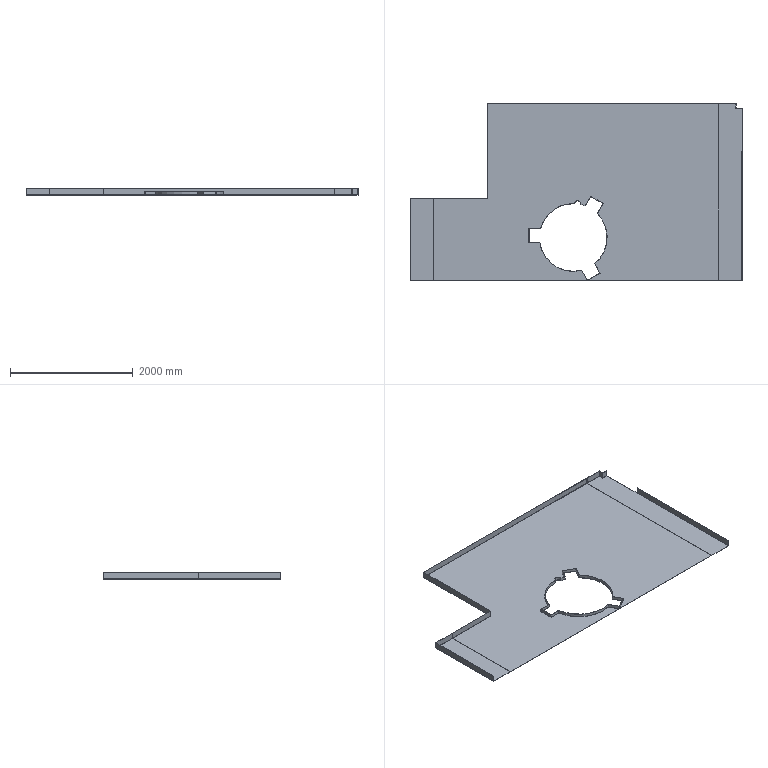Part | STEP file | PN_0043 checkered steel plate 4785x1464_Default<As Machined> | 8 solids | 100 faces | box 5405 x 2881 x 103 mm | volume 41382976 mm3 | plane 85 | cylinder 15 | commonest cylinder face diameters 1100 x8 1106 x4 100 x2 106 x1